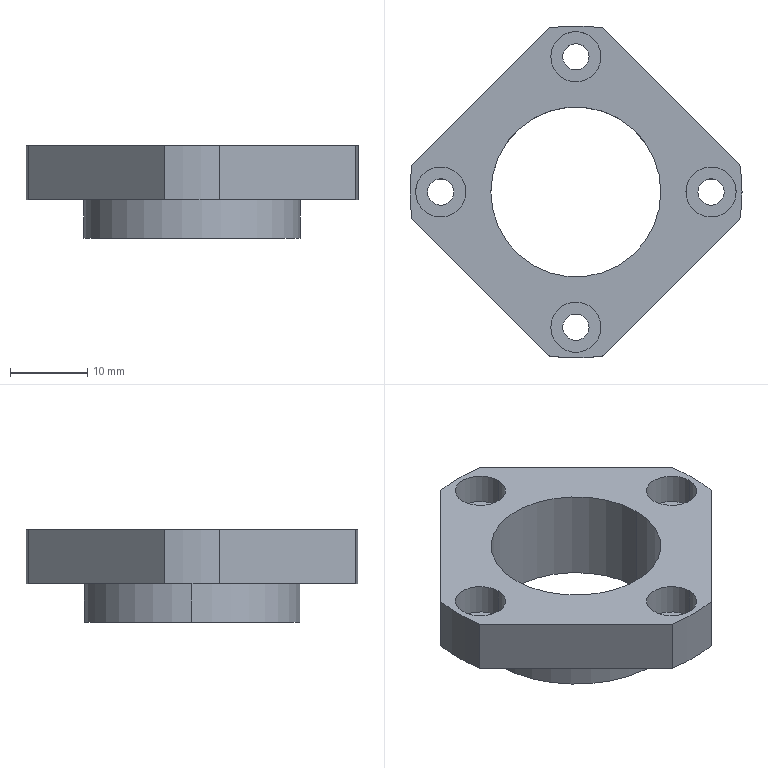Part | SolidWorks | features BaseBody 1 | 1 solid | 36 faces | box 43 x 43 x 12 mm | volume 6140 mm3 | cylinder 25 | plane 11 | commonest cylinder face diameters 3.4 x8 6.5 x8 43 x5 22 x2 28 x2
STEP:
#1=CARTESIAN_POINT('',(-11.,0.,-12.));
#2=VERTEX_POINT('',#1);
#3=CARTESIAN_POINT('',(11.,0.,-12.));
#4=VERTEX_POINT('',#3);
#5=CARTESIAN_POINT('',(0.,0.,-12.));
#6=DIRECTION('',(0.,0.,1.));
#7=DIRECTION('',(1.,0.,0.));
#8=AXIS2_PLACEMENT_3D('',#5,#6,#7);
#9=CIRCLE('',#8,11.);
#10=EDGE_CURVE('',#2,#4,#9,.T.);
#11=ORIENTED_EDGE('',*,*,#10,.F.);
#12=CARTESIAN_POINT('',(-11.,0.,0.));
#13=VERTEX_POINT('',#12);
#14=CARTESIAN_POINT('',(-11.,0.,-50.));
#15=DIRECTION('',(0.,0.,1.));
#16=VECTOR('',#15,1000.);
#17=LINE('',#14,#16);
#18=EDGE_CURVE('',#2,#13,#17,.T.);
#19=ORIENTED_EDGE('',*,*,#18,.T.);
#20=CARTESIAN_POINT('',(11.,0.,0.));
#21=VERTEX_POINT('',#20);
#22=CARTESIAN_POINT('',(0.,0.,0.));
#23=DIRECTION('',(0.,0.,-1.));
#24=DIRECTION('',(1.,0.,0.));
#25=AXIS2_PLACEMENT_3D('',#22,#23,#24);
#26=CIRCLE('',#25,11.);
#27=EDGE_CURVE('',#21,#13,#26,.T.);
#28=ORIENTED_EDGE('',*,*,#27,.F.);
#29=CARTESIAN_POINT('',(11.,0.,-50.));
#30=DIRECTION('',(0.,0.,1.));
#31=VECTOR('',#30,1000.);
#32=LINE('',#29,#31);
#33=EDGE_CURVE('',#4,#21,#32,.T.);
#34=ORIENTED_EDGE('',*,*,#33,.F.);
#35=EDGE_LOOP('',(#11,#19,#28,#34));
#36=FACE_OUTER_BOUND('',#35,.T.);
#37=CARTESIAN_POINT('',(0.,0.,-50.));
#38=DIRECTION('',(0.,0.,1.));
#39=DIRECTION('',(1.,0.,0.));
#40=AXIS2_PLACEMENT_3D('',#37,#38,#39);
#41=CYLINDRICAL_SURFACE('',#40,11.);
#42=ADVANCED_FACE('',(#36),#41,.F.);
#43=CARTESIAN_POINT('',(3.25,-17.5,0.));
#44=VERTEX_POINT('',#43);
#45=CARTESIAN_POINT('',(-3.25,-17.5,0.));
#46=VERTEX_POINT('',#45);
#47=CARTESIAN_POINT('',(0.,-17.5,0.));
#48=DIRECTION('',(0.,0.,-1.));
#49=DIRECTION('',(-1.,0.,0.));
#50=AXIS2_PLACEMENT_3D('',#47,#48,#49);
#51=CIRCLE('',#50,3.25);
#52=EDGE_CURVE('',#44,#46,#51,.T.);
#53=ORIENTED_EDGE('',*,*,#52,.F.);
#54=CARTESIAN_POINT('',(3.25,-17.5,-4.));
#55=VERTEX_POINT('',#54);
#56=CARTESIAN_POINT('',(3.25,-17.5,0.));
#57=DIRECTION('',(0.,0.,-1.));
#58=VECTOR('',#57,1000.);
#59=LINE('',#56,#58);
#60=EDGE_CURVE('',#44,#55,#59,.T.);
#61=ORIENTED_EDGE('',*,*,#60,.T.);
#62=CARTESIAN_POINT('',(-3.25,-17.5,-4.));
#63=VERTEX_POINT('',#62);
#64=CARTESIAN_POINT('',(0.,-17.5,-4.));
#65=DIRECTION('',(0.,0.,1.));
#66=DIRECTION('',(-1.,0.,0.));
#67=AXIS2_PLACEMENT_3D('',#64,#65,#66);
#68=CIRCLE('',#67,3.25);
#69=EDGE_CURVE('',#63,#55,#68,.T.);
#70=ORIENTED_EDGE('',*,*,#69,.F.);
#71=CARTESIAN_POINT('',(-3.25,-17.5,0.));
#72=DIRECTION('',(0.,0.,-1.));
#73=VECTOR('',#72,1000.);
#74=LINE('',#71,#73);
#75=EDGE_CURVE('',#46,#63,#74,.T.);
#76=ORIENTED_EDGE('',*,*,#75,.F.);
#77=EDGE_LOOP('',(#53,#61,#70,#76));
#78=FACE_OUTER_BOUND('',#77,.T.);
#79=CARTESIAN_POINT('',(0.,-17.5,0.));
#80=DIRECTION('',(0.,0.,-1.));
#81=DIRECTION('',(-1.,0.,0.));
#82=AXIS2_PLACEMENT_3D('',#79,#80,#81);
#83=CYLINDRICAL_SURFACE('',#82,3.25);
#84=ADVANCED_FACE('',(#78),#83,.F.);
#85=CARTESIAN_POINT('',(20.75,0.,0.));
#86=VERTEX_POINT('',#85);
#87=CARTESIAN_POINT('',(14.25,0.,0.));
#88=VERTEX_POINT('',#87);
#89=CARTESIAN_POINT('',(17.5,0.,0.));
#90=DIRECTION('',(0.,0.,-1.));
#91=DIRECTION('',(-1.,0.,0.));
#92=AXIS2_PLACEMENT_3D('',#89,#90,#91);
#93=CIRCLE('',#92,3.25);
#94=EDGE_CURVE('',#86,#88,#93,.T.);
#95=ORIENTED_EDGE('',*,*,#94,.F.);
#96=CARTESIAN_POINT('',(20.75,0.,-4.));
#97=VERTEX_POINT('',#96);
#98=CARTESIAN_POINT('',(20.75,0.,0.));
#99=DIRECTION('',(0.,0.,-1.));
#100=VECTOR('',#99,1000.);
#101=LINE('',#98,#100);
#102=EDGE_CURVE('',#86,#97,#101,.T.);
#103=ORIENTED_EDGE('',*,*,#102,.T.);
#104=CARTESIAN_POINT('',(14.25,0.,-4.));
#105=VERTEX_POINT('',#104);
#106=CARTESIAN_POINT('',(17.5,0.,-4.));
#107=DIRECTION('',(0.,0.,1.));
#108=DIRECTION('',(-1.,0.,0.));
#109=AXIS2_PLACEMENT_3D('',#106,#107,#108);
#110=CIRCLE('',#109,3.25);
#111=EDGE_CURVE('',#105,#97,#110,.T.);
#112=ORIENTED_EDGE('',*,*,#111,.F.);
#113=CARTESIAN_POINT('',(14.25,0.,0.));
#114=DIRECTION('',(0.,0.,-1.));
#115=VECTOR('',#114,1000.);
#116=LINE('',#113,#115);
#117=EDGE_CURVE('',#88,#105,#116,.T.);
#118=ORIENTED_EDGE('',*,*,#117,.F.);
#119=EDGE_LOOP('',(#95,#103,#112,#118));
#120=FACE_OUTER_BOUND('',#119,.T.);
#121=CARTESIAN_POINT('',(17.5,0.,0.));
#122=DIRECTION('',(0.,0.,-1.));
#123=DIRECTION('',(-1.,0.,0.));
#124=AXIS2_PLACEMENT_3D('',#121,#122,#123);
#125=CYLINDRICAL_SURFACE('',#124,3.25);
#126=ADVANCED_FACE('',(#120),#125,.F.);
#127=CARTESIAN_POINT('',(-20.75,0.,-4.));
#128=VERTEX_POINT('',#127);
#129=CARTESIAN_POINT('',(-14.25,0.,-4.));
#130=VERTEX_POINT('',#129);
#131=CARTESIAN_POINT('',(-17.5,0.,-4.));
#132=DIRECTION('',(0.,0.,1.));
#133=DIRECTION('',(1.,0.,0.));
#134=AXIS2_PLACEMENT_3D('',#131,#132,#133);
#135=CIRCLE('',#134,3.25);
#136=EDGE_CURVE('',#128,#130,#135,.T.);
#137=ORIENTED_EDGE('',*,*,#136,.F.);
#138=CARTESIAN_POINT('',(-20.75,0.,0.));
#139=VERTEX_POINT('',#138);
#140=CARTESIAN_POINT('',(-20.75,0.,-7.));
#141=DIRECTION('',(0.,0.,1.));
#142=VECTOR('',#141,1000.);
#143=LINE('',#140,#142);
#144=EDGE_CURVE('',#128,#139,#143,.T.);
#145=ORIENTED_EDGE('',*,*,#144,.T.);
#146=CARTESIAN_POINT('',(-14.25,0.,0.));
#147=VERTEX_POINT('',#146);
#148=CARTESIAN_POINT('',(-17.5,0.,0.));
#149=DIRECTION('',(0.,0.,-1.));
#150=DIRECTION('',(1.,0.,0.));
#151=AXIS2_PLACEMENT_3D('',#148,#149,#150);
#152=CIRCLE('',#151,3.25);
#153=EDGE_CURVE('',#147,#139,#152,.T.);
#154=ORIENTED_EDGE('',*,*,#153,.F.);
#155=CARTESIAN_POINT('',(-14.25,0.,-7.));
#156=DIRECTION('',(0.,0.,1.));
#157=VECTOR('',#156,1000.);
#158=LINE('',#155,#157);
#159=EDGE_CURVE('',#130,#147,#158,.T.);
#160=ORIENTED_EDGE('',*,*,#159,.F.);
#161=EDGE_LOOP('',(#137,#145,#154,#160));
#162=FACE_OUTER_BOUND('',#161,.T.);
#163=CARTESIAN_POINT('',(-17.5,0.,-7.));
#164=DIRECTION('',(0.,0.,1.));
#165=DIRECTION('',(1.,0.,0.));
#166=AXIS2_PLACEMENT_3D('',#163,#164,#165);
#167=CYLINDRICAL_SURFACE('',#166,3.25);
#168=ADVANCED_FACE('',(#162),#167,.F.);
#169=CARTESIAN_POINT('',(21.206,-3.543,-7.));
#170=VERTEX_POINT('',#169);
#171=CARTESIAN_POINT('',(21.5,0.,-7.));
#172=VERTEX_POINT('',#171);
#173=CARTESIAN_POINT('',(0.,0.,-7.));
#174=DIRECTION('',(0.,0.,1.));
#175=DIRECTION('',(1.,0.,0.));
#176=AXIS2_PLACEMENT_3D('',#173,#174,#175);
#177=CIRCLE('',#176,21.5);
#178=EDGE_CURVE('',#170,#172,#177,.T.);
#179=ORIENTED_EDGE('',*,*,#178,.T.);
#180=CARTESIAN_POINT('',(21.5,0.,0.));
#181=VERTEX_POINT('',#180);
#182=CARTESIAN_POINT('',(21.5,0.,-50.));
#183=DIRECTION('',(0.,0.,1.));
#184=VECTOR('',#183,1000.);
#185=LINE('',#182,#184);
#186=EDGE_CURVE('',#172,#181,#185,.T.);
#187=ORIENTED_EDGE('',*,*,#186,.T.);
#188=CARTESIAN_POINT('',(21.206,-3.543,0.));
#189=VERTEX_POINT('',#188);
#190=CARTESIAN_POINT('',(0.,0.,0.));
#191=DIRECTION('',(0.,0.,1.));
#192=DIRECTION('',(1.,0.,0.));
#193=AXIS2_PLACEMENT_3D('',#190,#191,#192);
#194=CIRCLE('',#193,21.5);
#195=EDGE_CURVE('',#189,#181,#194,.T.);
#196=ORIENTED_EDGE('',*,*,#195,.F.);
#197=CARTESIAN_POINT('',(21.206,-3.543,-50.));
#198=DIRECTION('',(0.,0.,-1.));
#199=VECTOR('',#198,1000.);
#200=LINE('',#197,#199);
#201=EDGE_CURVE('',#189,#170,#200,.T.);
#202=ORIENTED_EDGE('',*,*,#201,.T.);
#203=EDGE_LOOP('',(#179,#187,#196,#202));
#204=FACE_OUTER_BOUND('',#203,.T.);
#205=CARTESIAN_POINT('',(0.,0.,-50.));
#206=DIRECTION('',(0.,0.,1.));
#207=DIRECTION('',(1.,0.,0.));
#208=AXIS2_PLACEMENT_3D('',#205,#206,#207);
#209=CYLINDRICAL_SURFACE('',#208,21.5);
#210=ADVANCED_FACE('',(#204),#209,.T.);
#211=CARTESIAN_POINT('',(-3.25,17.5,-4.));
#212=VERTEX_POINT('',#211);
#213=CARTESIAN_POINT('',(3.25,17.5,-4.));
#214=VERTEX_POINT('',#213);
#215=CARTESIAN_POINT('',(0.,17.5,-4.));
#216=DIRECTION('',(0.,0.,1.));
#217=DIRECTION('',(1.,0.,0.));
#218=AXIS2_PLACEMENT_3D('',#215,#216,#217);
#219=CIRCLE('',#218,3.25);
#220=EDGE_CURVE('',#212,#214,#219,.T.);
#221=ORIENTED_EDGE('',*,*,#220,.F.);
#222=CARTESIAN_POINT('',(-3.25,17.5,0.));
#223=VERTEX_POINT('',#222);
#224=CARTESIAN_POINT('',(-3.25,17.5,-7.));
#225=DIRECTION('',(0.,0.,1.));
#226=VECTOR('',#225,1000.);
#227=LINE('',#224,#226);
#228=EDGE_CURVE('',#212,#223,#227,.T.);
#229=ORIENTED_EDGE('',*,*,#228,.T.);
#230=CARTESIAN_POINT('',(3.25,17.5,0.));
#231=VERTEX_POINT('',#230);
#232=CARTESIAN_POINT('',(0.,17.5,0.));
#233=DIRECTION('',(0.,0.,-1.));
#234=DIRECTION('',(1.,0.,0.));
#235=AXIS2_PLACEMENT_3D('',#232,#233,#234);
#236=CIRCLE('',#235,3.25);
#237=EDGE_CURVE('',#231,#223,#236,.T.);
#238=ORIENTED_EDGE('',*,*,#237,.F.);
#239=CARTESIAN_POINT('',(3.25,17.5,-7.));
#240=DIRECTION('',(0.,0.,1.));
#241=VECTOR('',#240,1000.);
#242=LINE('',#239,#241);
#243=EDGE_CURVE('',#214,#231,#242,.T.);
#244=ORIENTED_EDGE('',*,*,#243,.F.);
#245=EDGE_LOOP('',(#221,#229,#238,#244));
#246=FACE_OUTER_BOUND('',#245,.T.);
#247=CARTESIAN_POINT('',(0.,17.5,-7.));
#248=DIRECTION('',(0.,0.,1.));
#249=DIRECTION('',(1.,0.,0.));
#250=AXIS2_PLACEMENT_3D('',#247,#248,#249);
#251=CYLINDRICAL_SURFACE('',#250,3.25);
#252=ADVANCED_FACE('',(#246),#251,.F.);
#253=CARTESIAN_POINT('',(-14.,0.,-12.));
#254=VERTEX_POINT('',#253);
#255=CARTESIAN_POINT('',(14.,0.,-12.));
#256=VERTEX_POINT('',#255);
#257=CARTESIAN_POINT('',(0.,0.,-12.));
#258=DIRECTION('',(0.,0.,-1.));
#259=DIRECTION('',(1.,0.,0.));
#260=AXIS2_PLACEMENT_3D('',#257,#258,#259);
#261=CIRCLE('',#260,14.);
#262=EDGE_CURVE('',#254,#256,#261,.T.);
#263=ORIENTED_EDGE('',*,*,#262,.F.);
#264=CARTESIAN_POINT('',(-14.,0.,-7.));
#265=VERTEX_POINT('',#264);
#266=CARTESIAN_POINT('',(-14.,0.,-50.));
#267=DIRECTION('',(0.,0.,1.));
#268=VECTOR('',#267,1000.);
#269=LINE('',#266,#268);
#270=EDGE_CURVE('',#254,#265,#269,.T.);
#271=ORIENTED_EDGE('',*,*,#270,.T.);
#272=CARTESIAN_POINT('',(14.,0.,-7.));
#273=VERTEX_POINT('',#272);
#274=CARTESIAN_POINT('',(0.,0.,-7.));
#275=DIRECTION('',(0.,0.,-1.));
#276=DIRECTION('',(1.,0.,0.));
#277=AXIS2_PLACEMENT_3D('',#274,#275,#276);
#278=CIRCLE('',#277,14.);
#279=EDGE_CURVE('',#265,#273,#278,.T.);
#280=ORIENTED_EDGE('',*,*,#279,.T.);
#281=CARTESIAN_POINT('',(14.,0.,-50.));
#282=DIRECTION('',(0.,0.,1.));
#283=VECTOR('',#282,1000.);
#284=LINE('',#281,#283);
#285=EDGE_CURVE('',#256,#273,#284,.T.);
#286=ORIENTED_EDGE('',*,*,#285,.F.);
#287=EDGE_LOOP('',(#263,#271,#280,#286));
#288=FACE_OUTER_BOUND('',#287,.T.);
#289=CARTESIAN_POINT('',(0.,0.,-50.));
#290=DIRECTION('',(0.,0.,1.));
#291=DIRECTION('',(1.,0.,0.));
#292=AXIS2_PLACEMENT_3D('',#289,#290,#291);
#293=CYLINDRICAL_SURFACE('',#292,14.);
#294=ADVANCED_FACE('',(#288),#293,.T.);
#295=CARTESIAN_POINT('',(1.7,-17.5,-4.));
#296=VERTEX_POINT('',#295);
#297=CARTESIAN_POINT('',(-1.7,-17.5,-4.));
#298=VERTEX_POINT('',#297);
#299=CARTESIAN_POINT('',(0.,-17.5,-4.));
#300=DIRECTION('',(0.,0.,-1.));
#301=DIRECTION('',(-1.,0.,0.));
#302=AXIS2_PLACEMENT_3D('',#299,#300,#301);
#303=CIRCLE('',#302,1.7);
#304=EDGE_CURVE('',#296,#298,#303,.T.);
#305=ORIENTED_EDGE('',*,*,#304,.F.);
#306=CARTESIAN_POINT('',(1.7,-17.5,-7.));
#307=VERTEX_POINT('',#306);
#308=CARTESIAN_POINT('',(1.7,-17.5,0.));
#309=DIRECTION('',(0.,0.,-1.));
#310=VECTOR('',#309,1000.);
#311=LINE('',#308,#310);
#312=EDGE_CURVE('',#296,#307,#311,.T.);
#313=ORIENTED_EDGE('',*,*,#312,.T.);
#314=CARTESIAN_POINT('',(-1.7,-17.5,-7.));
#315=VERTEX_POINT('',#314);
#316=CARTESIAN_POINT('',(0.,-17.5,-7.));
#317=DIRECTION('',(0.,0.,1.));
#318=DIRECTION('',(-1.,0.,0.));
#319=AXIS2_PLACEMENT_3D('',#316,#317,#318);
#320=CIRCLE('',#319,1.7);
#321=EDGE_CURVE('',#315,#307,#320,.T.);
#322=ORIENTED_EDGE('',*,*,#321,.F.);
#323=CARTESIAN_POINT('',(-1.7,-17.5,0.));
#324=DIRECTION('',(0.,0.,-1.));
#325=VECTOR('',#324,1000.);
#326=LINE('',#323,#325);
#327=EDGE_CURVE('',#298,#315,#326,.T.);
#328=ORIENTED_EDGE('',*,*,#327,.F.);
#329=EDGE_LOOP('',(#305,#313,#322,#328));
#330=FACE_OUTER_BOUND('',#329,.T.);
#331=CARTESIAN_POINT('',(0.,-17.5,0.));
#332=DIRECTION('',(0.,0.,-1.));
#333=DIRECTION('',(-1.,0.,0.));
#334=AXIS2_PLACEMENT_3D('',#331,#332,#333);
#335=CYLINDRICAL_SURFACE('',#334,1.7);
#336=ADVANCED_FACE('',(#330),#335,.F.);
#337=CARTESIAN_POINT('',(19.2,0.,-4.));
#338=VERTEX_POINT('',#337);
#339=CARTESIAN_POINT('',(15.8,0.,-4.));
#340=VERTEX_POINT('',#339);
#341=CARTESIAN_POINT('',(17.5,0.,-4.));
#342=DIRECTION('',(0.,0.,-1.));
#343=DIRECTION('',(-1.,0.,0.));
#344=AXIS2_PLACEMENT_3D('',#341,#342,#343);
#345=CIRCLE('',#344,1.7);
#346=EDGE_CURVE('',#338,#340,#345,.T.);
#347=ORIENTED_EDGE('',*,*,#346,.F.);
#348=CARTESIAN_POINT('',(19.2,0.,-7.));
#349=VERTEX_POINT('',#348);
#350=CARTESIAN_POINT('',(19.2,0.,0.));
#351=DIRECTION('',(0.,0.,-1.));
#352=VECTOR('',#351,1000.);
#353=LINE('',#350,#352);
#354=EDGE_CURVE('',#338,#349,#353,.T.);
#355=ORIENTED_EDGE('',*,*,#354,.T.);
#356=CARTESIAN_POINT('',(15.8,0.,-7.));
#357=VERTEX_POINT('',#356);
#358=CARTESIAN_POINT('',(17.5,0.,-7.));
#359=DIRECTION('',(0.,0.,1.));
#360=DIRECTION('',(-1.,0.,0.));
#361=AXIS2_PLACEMENT_3D('',#358,#359,#360);
#362=CIRCLE('',#361,1.7);
#363=EDGE_CURVE('',#357,#349,#362,.T.);
#364=ORIENTED_EDGE('',*,*,#363,.F.);
#365=CARTESIAN_POINT('',(15.8,0.,0.));
#366=DIRECTION('',(0.,0.,-1.));
#367=VECTOR('',#366,1000.);
#368=LINE('',#365,#367);
#369=EDGE_CURVE('',#340,#357,#368,.T.);
#370=ORIENTED_EDGE('',*,*,#369,.F.);
#371=EDGE_LOOP('',(#347,#355,#364,#370));
#372=FACE_OUTER_BOUND('',#371,.T.);
#373=CARTESIAN_POINT('',(17.5,0.,0.));
#374=DIRECTION('',(0.,0.,-1.));
#375=DIRECTION('',(-1.,0.,0.));
#376=AXIS2_PLACEMENT_3D('',#373,#374,#375);
#377=CYLINDRICAL_SURFACE('',#376,1.7);
#378=ADVANCED_FACE('',(#372),#377,.F.);
#379=CARTESIAN_POINT('',(-19.2,0.,-7.));
#380=VERTEX_POINT('',#379);
#381=CARTESIAN_POINT('',(-15.8,0.,-7.));
#382=VERTEX_POINT('',#381);
#383=CARTESIAN_POINT('',(-17.5,0.,-7.));
#384=DIRECTION('',(0.,0.,1.));
#385=DIRECTION('',(1.,0.,0.));
#386=AXIS2_PLACEMENT_3D('',#383,#384,#385);
#387=CIRCLE('',#386,1.7);
#388=EDGE_CURVE('',#380,#382,#387,.T.);
#389=ORIENTED_EDGE('',*,*,#388,.F.);
#390=CARTESIAN_POINT('',(-19.2,0.,-4.));
#391=VERTEX_POINT('',#390);
#392=CARTESIAN_POINT('',(-19.2,0.,-7.));
#393=DIRECTION('',(0.,0.,1.));
#394=VECTOR('',#393,1000.);
#395=LINE('',#392,#394);
#396=EDGE_CURVE('',#380,#391,#395,.T.);
#397=ORIENTED_EDGE('',*,*,#396,.T.);
#398=CARTESIAN_POINT('',(-15.8,0.,-4.));
#399=VERTEX_POINT('',#398);
#400=CARTESIAN_POINT('',(-17.5,0.,-4.));
#401=DIRECTION('',(0.,0.,-1.));
#402=DIRECTION('',(1.,0.,0.));
#403=AXIS2_PLACEMENT_3D('',#400,#401,#402);
#404=CIRCLE('',#403,1.7);
#405=EDGE_CURVE('',#399,#391,#404,.T.);
#406=ORIENTED_EDGE('',*,*,#405,.F.);
#407=CARTESIAN_POINT('',(-15.8,0.,-7.));
#408=DIRECTION('',(0.,0.,1.));
#409=VECTOR('',#408,1000.);
#410=LINE('',#407,#409);
#411=EDGE_CURVE('',#382,#399,#410,.T.);
#412=ORIENTED_EDGE('',*,*,#411,.F.);
#413=EDGE_LOOP('',(#389,#397,#406,#412));
#414=FACE_OUTER_BOUND('',#413,.T.);
#415=CARTESIAN_POINT('',(-17.5,0.,-7.));
#416=DIRECTION('',(0.,0.,1.));
#417=DIRECTION('',(1.,0.,0.));
#418=AXIS2_PLACEMENT_3D('',#415,#416,#417);
#419=CYLINDRICAL_SURFACE('',#418,1.7);
#420=ADVANCED_FACE('',(#414),#419,.F.);
#421=CARTESIAN_POINT('',(-1.7,17.5,-7.));
#422=VERTEX_POINT('',#421);
#423=CARTESIAN_POINT('',(1.7,17.5,-7.));
#424=VERTEX_POINT('',#423);
#425=CARTESIAN_POINT('',(0.,17.5,-7.));
#426=DIRECTION('',(0.,0.,1.));
#427=DIRECTION('',(1.,0.,0.));
#428=AXIS2_PLACEMENT_3D('',#425,#426,#427);
#429=CIRCLE('',#428,1.7);
#430=EDGE_CURVE('',#422,#424,#429,.T.);
#431=ORIENTED_EDGE('',*,*,#430,.F.);
#432=CARTESIAN_POINT('',(-1.7,17.5,-4.));
#433=VERTEX_POINT('',#432);
#434=CARTESIAN_POINT('',(-1.7,17.5,-7.));
#435=DIRECTION('',(0.,0.,1.));
#436=VECTOR('',#435,1000.);
#437=LINE('',#434,#436);
#438=EDGE_CURVE('',#422,#433,#437,.T.);
#439=ORIENTED_EDGE('',*,*,#438,.T.);
#440=CARTESIAN_POINT('',(1.7,17.5,-4.));
#441=VERTEX_POINT('',#440);
#442=CARTESIAN_POINT('',(0.,17.5,-4.));
#443=DIRECTION('',(0.,0.,-1.));
#444=DIRECTION('',(1.,0.,0.));
#445=AXIS2_PLACEMENT_3D('',#442,#443,#444);
#446=CIRCLE('',#445,1.7);
#447=EDGE_CURVE('',#441,#433,#446,.T.);
#448=ORIENTED_EDGE('',*,*,#447,.F.);
#449=CARTESIAN_POINT('',(1.7,17.5,-7.));
#450=DIRECTION('',(0.,0.,1.));
#451=VECTOR('',#450,1000.);
#452=LINE('',#449,#451);
#453=EDGE_CURVE('',#424,#441,#452,.T.);
#454=ORIENTED_EDGE('',*,*,#453,.F.);
#455=EDGE_LOOP('',(#431,#439,#448,#454));
#456=FACE_OUTER_BOUND('',#455,.T.);
#457=CARTESIAN_POINT('',(0.,17.5,-7.));
#458=DIRECTION('',(0.,0.,1.));
#459=DIRECTION('',(1.,0.,0.));
#460=AXIS2_PLACEMENT_3D('',#457,#458,#459);
#461=CYLINDRICAL_SURFACE('',#460,1.7);
#462=ADVANCED_FACE('',(#456),#461,.F.);
#463=ORIENTED_EDGE('',*,*,#18,.F.);
#464=CARTESIAN_POINT('',(0.,0.,-12.));
#465=DIRECTION('',(0.,0.,1.));
#466=DIRECTION('',(1.,0.,0.));
#467=AXIS2_PLACEMENT_3D('',#464,#465,#466);
#468=CIRCLE('',#467,11.);
#469=EDGE_CURVE('',#4,#2,#468,.T.);
#470=ORIENTED_EDGE('',*,*,#469,.F.);
#471=ORIENTED_EDGE('',*,*,#33,.T.);
#472=CARTESIAN_POINT('',(0.,0.,0.));
#473=DIRECTION('',(0.,0.,-1.));
#474=DIRECTION('',(1.,0.,0.));
#475=AXIS2_PLACEMENT_3D('',#472,#473,#474);
#476=CIRCLE('',#475,11.);
#477=EDGE_CURVE('',#13,#21,#476,.T.);
#478=ORIENTED_EDGE('',*,*,#477,.F.);
#479=EDGE_LOOP('',(#463,#470,#471,#478));
#480=FACE_OUTER_BOUND('',#479,.T.);
#481=CARTESIAN_POINT('',(0.,0.,-50.));
#482=DIRECTION('',(0.,0.,1.));
#483=DIRECTION('',(1.,0.,0.));
#484=AXIS2_PLACEMENT_3D('',#481,#482,#483);
#485=CYLINDRICAL_SURFACE('',#484,11.);
#486=ADVANCED_FACE('',(#480),#485,.F.);
#487=CARTESIAN_POINT('',(0.,-17.5,0.));
#488=DIRECTION('',(0.,0.,-1.));
#489=DIRECTION('',(-1.,0.,0.));
#490=AXIS2_PLACEMENT_3D('',#487,#488,#489);
#491=CIRCLE('',#490,3.25);
#492=EDGE_CURVE('',#46,#44,#491,.T.);
#493=ORIENTED_EDGE('',*,*,#492,.T.);
#494=ORIENTED_EDGE('',*,*,#52,.T.);
#495=EDGE_LOOP('',(#493,#494));
#496=FACE_BOUND('',#495,.T.);
#497=CARTESIAN_POINT('',(17.5,0.,0.));
#498=DIRECTION('',(0.,0.,-1.));
#499=DIRECTION('',(-1.,0.,0.));
#500=AXIS2_PLACEMENT_3D('',#497,#498,#499);
#501=CIRCLE('',#500,3.25);
#502=EDGE_CURVE('',#88,#86,#501,.T.);
#503=ORIENTED_EDGE('',*,*,#502,.T.);
#504=ORIENTED_EDGE('',*,*,#94,.T.);
#505=EDGE_LOOP('',(#503,#504));
#506=FACE_BOUND('',#505,.T.);
#507=ORIENTED_EDGE('',*,*,#153,.T.);
#508=CARTESIAN_POINT('',(-17.5,0.,0.));
#509=DIRECTION('',(0.,0.,-1.));
#510=DIRECTION('',(1.,0.,0.));
#511=AXIS2_PLACEMENT_3D('',#508,#509,#510);
#512=CIRCLE('',#511,3.25);
#513=EDGE_CURVE('',#139,#147,#512,.T.);
#514=ORIENTED_EDGE('',*,*,#513,.T.);
#515=EDGE_LOOP('',(#507,#514));
#516=FACE_BOUND('',#515,.T.);
#517=CARTESIAN_POINT('',(-21.206,-3.543,0.));
#518=VERTEX_POINT('',#517);
#519=CARTESIAN_POINT('',(-3.543,-21.206,0.));
#520=VERTEX_POINT('',#519);
#521=CARTESIAN_POINT('',(-21.206,-3.543,0.));
#522=DIRECTION('',(0.7071,-0.7071,0.));
#523=VECTOR('',#522,1000.);
#524=LINE('',#521,#523);
#525=EDGE_CURVE('',#518,#520,#524,.T.);
#526=ORIENTED_EDGE('',*,*,#525,.T.);
#527=CARTESIAN_POINT('',(3.543,-21.206,0.));
#528=VERTEX_POINT('',#527);
#529=CARTESIAN_POINT('',(0.,0.,0.));
#530=DIRECTION('',(0.,0.,1.));
#531=DIRECTION('',(1.,0.,0.));
#532=AXIS2_PLACEMENT_3D('',#529,#530,#531);
#533=CIRCLE('',#532,21.5);
#534=EDGE_CURVE('',#520,#528,#533,.T.);
#535=ORIENTED_EDGE('',*,*,#534,.T.);
#536=CARTESIAN_POINT('',(3.543,-21.206,0.));
#537=DIRECTION('',(0.7071,0.7071,0.));
#538=VECTOR('',#537,1000.);
#539=LINE('',#536,#538);
#540=EDGE_CURVE('',#528,#189,#539,.T.);
#541=ORIENTED_EDGE('',*,*,#540,.T.);
#542=ORIENTED_EDGE('',*,*,#195,.T.);
#543=CARTESIAN_POINT('',(21.206,3.543,0.));
#544=VERTEX_POINT('',#543);
#545=CARTESIAN_POINT('',(0.,0.,0.));
#546=DIRECTION('',(0.,0.,1.));
#547=DIRECTION('',(1.,0.,0.));
#548=AXIS2_PLACEMENT_3D('',#545,#546,#547);
#549=CIRCLE('',#548,21.5);
#550=EDGE_CURVE('',#181,#544,#549,.T.);
#551=ORIENTED_EDGE('',*,*,#550,.T.);
#552=CARTESIAN_POINT('',(3.543,21.206,0.));
#553=VERTEX_POINT('',#552);
#554=CARTESIAN_POINT('',(21.206,3.543,0.));
#555=DIRECTION('',(-0.7071,0.7071,0.));
#556=VECTOR('',#555,1000.);
#557=LINE('',#554,#556);
#558=EDGE_CURVE('',#544,#553,#557,.T.);
#559=ORIENTED_EDGE('',*,*,#558,.T.);
#560=CARTESIAN_POINT('',(-3.543,21.206,0.));
#561=VERTEX_POINT('',#560);
#562=CARTESIAN_POINT('',(0.,0.,0.));
#563=DIRECTION('',(0.,0.,1.));
#564=DIRECTION('',(1.,0.,0.));
#565=AXIS2_PLACEMENT_3D('',#562,#563,#564);
#566=CIRCLE('',#565,21.5);
#567=EDGE_CURVE('',#553,#561,#566,.T.);
#568=ORIENTED_EDGE('',*,*,#567,.T.);
#569=CARTESIAN_POINT('',(-21.206,3.543,0.));
#570=VERTEX_POINT('',#569);
#571=CARTESIAN_POINT('',(-3.543,21.206,0.));
#572=DIRECTION('',(-0.7071,-0.7071,0.));
#573=VECTOR('',#572,1000.);
#574=LINE('',#571,#573);
#575=EDGE_CURVE('',#561,#570,#574,.T.);
#576=ORIENTED_EDGE('',*,*,#575,.T.);
#577=CARTESIAN_POINT('',(0.,0.,0.));
#578=DIRECTION('',(0.,0.,1.));
#579=DIRECTION('',(1.,0.,0.));
#580=AXIS2_PLACEMENT_3D('',#577,#578,#579);
#581=CIRCLE('',#580,21.5);
#582=EDGE_CURVE('',#570,#518,#581,.T.);
#583=ORIENTED_EDGE('',*,*,#582,.T.);
#584=EDGE_LOOP('',(#526,#535,#541,#542,#551,#559,#568,#576,#583));
#585=FACE_OUTER_BOUND('',#584,.T.);
#586=ORIENTED_EDGE('',*,*,#237,.T.);
#587=CARTESIAN_POINT('',(0.,17.5,0.));
#588=DIRECTION('',(0.,0.,-1.));
#589=DIRECTION('',(1.,0.,0.));
#590=AXIS2_PLACEMENT_3D('',#587,#588,#589);
#591=CIRCLE('',#590,3.25);
#592=EDGE_CURVE('',#223,#231,#591,.T.);
#593=ORIENTED_EDGE('',*,*,#592,.T.);
#594=EDGE_LOOP('',(#586,#593));
#595=FACE_BOUND('',#594,.T.);
#596=ORIENTED_EDGE('',*,*,#27,.T.);
#597=ORIENTED_EDGE('',*,*,#477,.T.);
#598=EDGE_LOOP('',(#596,#597));
#599=FACE_BOUND('',#598,.T.);
#600=CARTESIAN_POINT('',(0.,21.5,0.));
#601=DIRECTION('',(0.,0.,1.));
#602=DIRECTION('',(1.,0.,0.));
#603=AXIS2_PLACEMENT_3D('',#600,#601,#602);
#604=PLANE('',#603);
#605=ADVANCED_FACE('',(#496,#506,#516,#585,#595,#599),#604,.T.);
#606=ORIENTED_EDGE('',*,*,#469,.T.);
#607=ORIENTED_EDGE('',*,*,#10,.T.);
#608=EDGE_LOOP('',(#606,#607));
#609=FACE_BOUND('',#608,.T.);
#610=CARTESIAN_POINT('',(0.,0.,-12.));
#611=DIRECTION('',(0.,0.,-1.));
#612=DIRECTION('',(1.,0.,0.));
#613=AXIS2_PLACEMENT_3D('',#610,#611,#612);
#614=CIRCLE('',#613,14.);
#615=EDGE_CURVE('',#256,#254,#614,.T.);
#616=ORIENTED_EDGE('',*,*,#615,.T.);
#617=ORIENTED_EDGE('',*,*,#262,.T.);
#618=EDGE_LOOP('',(#616,#617));
#619=FACE_OUTER_BOUND('',#618,.T.);
#620=CARTESIAN_POINT('',(0.,11.,-12.));
#621=DIRECTION('',(0.,0.,-1.));
#622=DIRECTION('',(-1.,0.,0.));
#623=AXIS2_PLACEMENT_3D('',#620,#621,#622);
#624=PLANE('',#623);
#625=ADVANCED_FACE('',(#609,#619),#624,.T.);
#626=ORIENTED_EDGE('',*,*,#60,.F.);
#627=ORIENTED_EDGE('',*,*,#492,.F.);
#628=ORIENTED_EDGE('',*,*,#75,.T.);
#629=CARTESIAN_POINT('',(0.,-17.5,-4.));
#630=DIRECTION('',(0.,0.,1.));
#631=DIRECTION('',(-1.,0.,0.));
#632=AXIS2_PLACEMENT_3D('',#629,#630,#631);
#633=CIRCLE('',#632,3.25);
#634=EDGE_CURVE('',#55,#63,#633,.T.);
#635=ORIENTED_EDGE('',*,*,#634,.F.);
#636=EDGE_LOOP('',(#626,#627,#628,#635));
#637=FACE_OUTER_BOUND('',#636,.T.);
#638=CARTESIAN_POINT('',(0.,-17.5,0.));
#639=DIRECTION('',(0.,0.,-1.));
#640=DIRECTION('',(-1.,0.,0.));
#641=AXIS2_PLACEMENT_3D('',#638,#639,#640);
#642=CYLINDRICAL_SURFACE('',#641,3.25);
#643=ADVANCED_FACE('',(#637),#642,.F.);
#644=ORIENTED_EDGE('',*,*,#102,.F.);
#645=ORIENTED_EDGE('',*,*,#502,.F.);
#646=ORIENTED_EDGE('',*,*,#117,.T.);
#647=CARTESIAN_POINT('',(17.5,0.,-4.));
#648=DIRECTION('',(0.,0.,1.));
#649=DIRECTION('',(-1.,0.,0.));
#650=AXIS2_PLACEMENT_3D('',#647,#648,#649);
#651=CIRCLE('',#650,3.25);
#652=EDGE_CURVE('',#97,#105,#651,.T.);
#653=ORIENTED_EDGE('',*,*,#652,.F.);
#654=EDGE_LOOP('',(#644,#645,#646,#653));
#655=FACE_OUTER_BOUND('',#654,.T.);
#656=CARTESIAN_POINT('',(17.5,0.,0.));
#657=DIRECTION('',(0.,0.,-1.));
#658=DIRECTION('',(-1.,0.,0.));
#659=AXIS2_PLACEMENT_3D('',#656,#657,#658);
#660=CYLINDRICAL_SURFACE('',#659,3.25);
#661=ADVANCED_FACE('',(#655),#660,.F.);
#662=ORIENTED_EDGE('',*,*,#144,.F.);
#663=CARTESIAN_POINT('',(-17.5,0.,-4.));
#664=DIRECTION('',(0.,0.,1.));
#665=DIRECTION('',(1.,0.,0.));
#666=AXIS2_PLACEMENT_3D('',#663,#664,#665);
#667=CIRCLE('',#666,3.25);
#668=EDGE_CURVE('',#130,#128,#667,.T.);
#669=ORIENTED_EDGE('',*,*,#668,.F.);
#670=ORIENTED_EDGE('',*,*,#159,.T.);
#671=ORIENTED_EDGE('',*,*,#513,.F.);
#672=EDGE_LOOP('',(#662,#669,#670,#671));
#673=FACE_OUTER_BOUND('',#672,.T.);
#674=CARTESIAN_POINT('',(-17.5,0.,-7.));
#675=DIRECTION('',(0.,0.,1.));
#676=DIRECTION('',(1.,0.,0.));
#677=AXIS2_PLACEMENT_3D('',#674,#675,#676);
#678=CYLINDRICAL_SURFACE('',#677,3.25);
#679=ADVANCED_FACE('',(#673),#678,.F.);
#680=CARTESIAN_POINT('',(-3.543,-21.206,-7.));
#681=VERTEX_POINT('',#680);
#682=CARTESIAN_POINT('',(-3.543,-21.206,-50.));
#683=DIRECTION('',(0.,0.,-1.));
#684=VECTOR('',#683,1000.);
#685=LINE('',#682,#684);
#686=EDGE_CURVE('',#520,#681,#685,.T.);
#687=ORIENTED_EDGE('',*,*,#686,.T.);
#688=CARTESIAN_POINT('',(3.543,-21.206,-7.));
#689=VERTEX_POINT('',#688);
#690=CARTESIAN_POINT('',(0.,0.,-7.));
#691=DIRECTION('',(0.,0.,1.));
#692=DIRECTION('',(1.,0.,0.));
#693=AXIS2_PLACEMENT_3D('',#690,#691,#692);
#694=CIRCLE('',#693,21.5);
#695=EDGE_CURVE('',#681,#689,#694,.T.);
#696=ORIENTED_EDGE('',*,*,#695,.T.);
#697=CARTESIAN_POINT('',(3.543,-21.206,-50.));
#698=DIRECTION('',(0.,0.,1.));
#699=VECTOR('',#698,1000.);
#700=LINE('',#697,#699);
#701=EDGE_CURVE('',#689,#528,#700,.T.);
#702=ORIENTED_EDGE('',*,*,#701,.T.);
#703=ORIENTED_EDGE('',*,*,#534,.F.);
#704=EDGE_LOOP('',(#687,#696,#702,#703));
#705=FACE_OUTER_BOUND('',#704,.T.);
#706=CARTESIAN_POINT('',(0.,0.,-50.));
#707=DIRECTION('',(0.,0.,1.));
#708=DIRECTION('',(1.,0.,0.));
#709=AXIS2_PLACEMENT_3D('',#706,#707,#708);
#710=CYLINDRICAL_SURFACE('',#709,21.5);
#711=ADVANCED_FACE('',(#705),#710,.T.);
#712=CARTESIAN_POINT('',(-21.206,-3.543,-7.));
#713=VERTEX_POINT('',#712);
#714=CARTESIAN_POINT('',(-21.206,-3.543,-7.));
#715=DIRECTION('',(0.,0.,1.));
#716=VECTOR('',#715,1000.);
#717=LINE('',#714,#716);
#718=EDGE_CURVE('',#713,#518,#717,.T.);
#719=ORIENTED_EDGE('',*,*,#718,.F.);
#720=CARTESIAN_POINT('',(-3.543,-21.206,-7.));
#721=DIRECTION('',(-0.7071,0.7071,0.));
#722=VECTOR('',#721,1000.);
#723=LINE('',#720,#722);
#724=EDGE_CURVE('',#681,#713,#723,.T.);
#725=ORIENTED_EDGE('',*,*,#724,.F.);
#726=ORIENTED_EDGE('',*,*,#686,.F.);
#727=ORIENTED_EDGE('',*,*,#525,.F.);
#728=EDGE_LOOP('',(#719,#725,#726,#727));
#729=FACE_OUTER_BOUND('',#728,.T.);
#730=CARTESIAN_POINT('',(-3.543,-21.206,-7.));
#731=DIRECTION('',(0.7071,0.7071,0.));
#732=DIRECTION('',(-0.7071,0.7071,0.));
#733=AXIS2_PLACEMENT_3D('',#730,#731,#732);
#734=PLANE('',#733);
#735=ADVANCED_FACE('',(#729),#734,.F.);
#736=CARTESIAN_POINT('',(-21.206,3.543,-7.));
#737=VERTEX_POINT('',#736);
#738=CARTESIAN_POINT('',(-21.206,3.543,-50.));
#739=DIRECTION('',(0.,0.,-1.));
#740=VECTOR('',#739,1000.);
#741=LINE('',#738,#740);
#742=EDGE_CURVE('',#570,#737,#741,.T.);
#743=ORIENTED_EDGE('',*,*,#742,.T.);
#744=CARTESIAN_POINT('',(0.,0.,-7.));
#745=DIRECTION('',(0.,0.,1.));
#746=DIRECTION('',(1.,0.,0.));
#747=AXIS2_PLACEMENT_3D('',#744,#745,#746);
#748=CIRCLE('',#747,21.5);
#749=EDGE_CURVE('',#737,#713,#748,.T.);
#750=ORIENTED_EDGE('',*,*,#749,.T.);
#751=ORIENTED_EDGE('',*,*,#718,.T.);
#752=ORIENTED_EDGE('',*,*,#582,.F.);
#753=EDGE_LOOP('',(#743,#750,#751,#752));
#754=FACE_OUTER_BOUND('',#753,.T.);
#755=CARTESIAN_POINT('',(0.,0.,-50.));
#756=DIRECTION('',(0.,0.,1.));
#757=DIRECTION('',(1.,0.,0.));
#758=AXIS2_PLACEMENT_3D('',#755,#756,#757);
#759=CYLINDRICAL_SURFACE('',#758,21.5);
#760=ADVANCED_FACE('',(#754),#759,.T.);
#761=CARTESIAN_POINT('',(-3.543,21.206,-7.));
#762=VERTEX_POINT('',#761);
#763=CARTESIAN_POINT('',(-3.543,21.206,-7.));
#764=DIRECTION('',(0.,0.,1.));
#765=VECTOR('',#764,1000.);
#766=LINE('',#763,#765);
#767=EDGE_CURVE('',#762,#561,#766,.T.);
#768=ORIENTED_EDGE('',*,*,#767,.F.);
#769=CARTESIAN_POINT('',(-21.206,3.543,-7.));
#770=DIRECTION('',(0.7071,0.7071,0.));
#771=VECTOR('',#770,1000.);
#772=LINE('',#769,#771);
#773=EDGE_CURVE('',#737,#762,#772,.T.);
#774=ORIENTED_EDGE('',*,*,#773,.F.);
#775=ORIENTED_EDGE('',*,*,#742,.F.);
#776=ORIENTED_EDGE('',*,*,#575,.F.);
#777=EDGE_LOOP('',(#768,#774,#775,#776));
#778=FACE_OUTER_BOUND('',#777,.T.);
#779=CARTESIAN_POINT('',(-21.206,3.543,-7.));
#780=DIRECTION('',(0.7071,-0.7071,0.));
#781=DIRECTION('',(0.7071,0.7071,0.));
#782=AXIS2_PLACEMENT_3D('',#779,#780,#781);
#783=PLANE('',#782);
#784=ADVANCED_FACE('',(#778),#783,.F.);
#785=CARTESIAN_POINT('',(3.543,21.206,-7.));
#786=VERTEX_POINT('',#785);
#787=CARTESIAN_POINT('',(3.543,21.206,-50.));
#788=DIRECTION('',(0.,0.,-1.));
#789=VECTOR('',#788,1000.);
#790=LINE('',#787,#789);
#791=EDGE_CURVE('',#553,#786,#790,.T.);
#792=ORIENTED_EDGE('',*,*,#791,.T.);
#793=CARTESIAN_POINT('',(0.,0.,-7.));
#794=DIRECTION('',(0.,0.,1.));
#795=DIRECTION('',(1.,0.,0.));
#796=AXIS2_PLACEMENT_3D('',#793,#794,#795);
#797=CIRCLE('',#796,21.5);
#798=EDGE_CURVE('',#786,#762,#797,.T.);
#799=ORIENTED_EDGE('',*,*,#798,.T.);
#800=ORIENTED_EDGE('',*,*,#767,.T.);
#801=ORIENTED_EDGE('',*,*,#567,.F.);
#802=EDGE_LOOP('',(#792,#799,#800,#801));
#803=FACE_OUTER_BOUND('',#802,.T.);
#804=CARTESIAN_POINT('',(0.,0.,-50.));
#805=DIRECTION('',(0.,0.,1.));
#806=DIRECTION('',(1.,0.,0.));
#807=AXIS2_PLACEMENT_3D('',#804,#805,#806);
#808=CYLINDRICAL_SURFACE('',#807,21.5);
#809=ADVANCED_FACE('',(#803),#808,.T.);
#810=CARTESIAN_POINT('',(21.206,3.543,-7.));
#811=VERTEX_POINT('',#810);
#812=CARTESIAN_POINT('',(21.206,3.543,-7.));
#813=DIRECTION('',(0.,0.,1.));
#814=VECTOR('',#813,1000.);
#815=LINE('',#812,#814);
#816=EDGE_CURVE('',#811,#544,#815,.T.);
#817=ORIENTED_EDGE('',*,*,#816,.F.);
#818=CARTESIAN_POINT('',(3.543,21.206,-7.));
#819=DIRECTION('',(0.7071,-0.7071,0.));
#820=VECTOR('',#819,1000.);
#821=LINE('',#818,#820);
#822=EDGE_CURVE('',#786,#811,#821,.T.);
#823=ORIENTED_EDGE('',*,*,#822,.F.);
#824=ORIENTED_EDGE('',*,*,#791,.F.);
#825=ORIENTED_EDGE('',*,*,#558,.F.);
#826=EDGE_LOOP('',(#817,#823,#824,#825));
#827=FACE_OUTER_BOUND('',#826,.T.);
#828=CARTESIAN_POINT('',(3.543,21.206,-7.));
#829=DIRECTION('',(-0.7071,-0.7071,0.));
#830=DIRECTION('',(0.7071,-0.7071,0.));
#831=AXIS2_PLACEMENT_3D('',#828,#829,#830);
#832=PLANE('',#831);
#833=ADVANCED_FACE('',(#827),#832,.F.);
#834=ORIENTED_EDGE('',*,*,#186,.F.);
#835=CARTESIAN_POINT('',(0.,0.,-7.));
#836=DIRECTION('',(0.,0.,1.));
#837=DIRECTION('',(1.,0.,0.));
#838=AXIS2_PLACEMENT_3D('',#835,#836,#837);
#839=CIRCLE('',#838,21.5);
#840=EDGE_CURVE('',#172,#811,#839,.T.);
#841=ORIENTED_EDGE('',*,*,#840,.T.);
#842=ORIENTED_EDGE('',*,*,#816,.T.);
#843=ORIENTED_EDGE('',*,*,#550,.F.);
#844=EDGE_LOOP('',(#834,#841,#842,#843));
#845=FACE_OUTER_BOUND('',#844,.T.);
#846=CARTESIAN_POINT('',(0.,0.,-50.));
#847=DIRECTION('',(0.,0.,1.));
#848=DIRECTION('',(1.,0.,0.));
#849=AXIS2_PLACEMENT_3D('',#846,#847,#848);
#850=CYLINDRICAL_SURFACE('',#849,21.5);
#851=ADVANCED_FACE('',(#845),#850,.T.);
#852=ORIENTED_EDGE('',*,*,#701,.F.);
#853=CARTESIAN_POINT('',(21.206,-3.543,-7.));
#854=DIRECTION('',(-0.7071,-0.7071,0.));
#855=VECTOR('',#854,1000.);
#856=LINE('',#853,#855);
#857=EDGE_CURVE('',#170,#689,#856,.T.);
#858=ORIENTED_EDGE('',*,*,#857,.F.);
#859=ORIENTED_EDGE('',*,*,#201,.F.);
#860=ORIENTED_EDGE('',*,*,#540,.F.);
#861=EDGE_LOOP('',(#852,#858,#859,#860));
#862=FACE_OUTER_BOUND('',#861,.T.);
#863=CARTESIAN_POINT('',(21.206,-3.543,-7.));
#864=DIRECTION('',(-0.7071,0.7071,0.));
#865=DIRECTION('',(-0.7071,-0.7071,0.));
#866=AXIS2_PLACEMENT_3D('',#863,#864,#865);
#867=PLANE('',#866);
#868=ADVANCED_FACE('',(#862),#867,.F.);
#869=ORIENTED_EDGE('',*,*,#228,.F.);
#870=CARTESIAN_POINT('',(0.,17.5,-4.));
#871=DIRECTION('',(0.,0.,1.));
#872=DIRECTION('',(1.,0.,0.));
#873=AXIS2_PLACEMENT_3D('',#870,#871,#872);
#874=CIRCLE('',#873,3.25);
#875=EDGE_CURVE('',#214,#212,#874,.T.);
#876=ORIENTED_EDGE('',*,*,#875,.F.);
#877=ORIENTED_EDGE('',*,*,#243,.T.);
#878=ORIENTED_EDGE('',*,*,#592,.F.);
#879=EDGE_LOOP('',(#869,#876,#877,#878));
#880=FACE_OUTER_BOUND('',#879,.T.);
#881=CARTESIAN_POINT('',(0.,17.5,-7.));
#882=DIRECTION('',(0.,0.,1.));
#883=DIRECTION('',(1.,0.,0.));
#884=AXIS2_PLACEMENT_3D('',#881,#882,#883);
#885=CYLINDRICAL_SURFACE('',#884,3.25);
#886=ADVANCED_FACE('',(#880),#885,.F.);
#887=ORIENTED_EDGE('',*,*,#270,.F.);
#888=ORIENTED_EDGE('',*,*,#615,.F.);
#889=ORIENTED_EDGE('',*,*,#285,.T.);
#890=CARTESIAN_POINT('',(0.,0.,-7.));
#891=DIRECTION('',(0.,0.,-1.));
#892=DIRECTION('',(1.,0.,0.));
#893=AXIS2_PLACEMENT_3D('',#890,#891,#892);
#894=CIRCLE('',#893,14.);
#895=EDGE_CURVE('',#273,#265,#894,.T.);
#896=ORIENTED_EDGE('',*,*,#895,.T.);
#897=EDGE_LOOP('',(#887,#888,#889,#896));
#898=FACE_OUTER_BOUND('',#897,.T.);
#899=CARTESIAN_POINT('',(0.,0.,-50.));
#900=DIRECTION('',(0.,0.,1.));
#901=DIRECTION('',(1.,0.,0.));
#902=AXIS2_PLACEMENT_3D('',#899,#900,#901);
#903=CYLINDRICAL_SURFACE('',#902,14.);
#904=ADVANCED_FACE('',(#898),#903,.T.);
#905=CARTESIAN_POINT('',(0.,-17.5,-4.));
#906=DIRECTION('',(0.,0.,-1.));
#907=DIRECTION('',(-1.,0.,0.));
#908=AXIS2_PLACEMENT_3D('',#905,#906,#907);
#909=CIRCLE('',#908,1.7);
#910=EDGE_CURVE('',#298,#296,#909,.T.);
#911=ORIENTED_EDGE('',*,*,#910,.T.);
#912=ORIENTED_EDGE('',*,*,#304,.T.);
#913=EDGE_LOOP('',(#911,#912));
#914=FACE_BOUND('',#913,.T.);
#915=ORIENTED_EDGE('',*,*,#69,.T.);
#916=ORIENTED_EDGE('',*,*,#634,.T.);
#917=EDGE_LOOP('',(#915,#916));
#918=FACE_OUTER_BOUND('',#917,.T.);
#919=CARTESIAN_POINT('',(0.,-19.2,-4.));
#920=DIRECTION('',(0.,0.,1.));
#921=DIRECTION('',(1.,0.,0.));
#922=AXIS2_PLACEMENT_3D('',#919,#920,#921);
#923=PLANE('',#922);
#924=ADVANCED_FACE('',(#914,#918),#923,.T.);
#925=CARTESIAN_POINT('',(17.5,0.,-4.));
#926=DIRECTION('',(0.,0.,-1.));
#927=DIRECTION('',(-1.,0.,0.));
#928=AXIS2_PLACEMENT_3D('',#925,#926,#927);
#929=CIRCLE('',#928,1.7);
#930=EDGE_CURVE('',#340,#338,#929,.T.);
#931=ORIENTED_EDGE('',*,*,#930,.T.);
#932=ORIENTED_EDGE('',*,*,#346,.T.);
#933=EDGE_LOOP('',(#931,#932));
#934=FACE_BOUND('',#933,.T.);
#935=ORIENTED_EDGE('',*,*,#111,.T.);
#936=ORIENTED_EDGE('',*,*,#652,.T.);
#937=EDGE_LOOP('',(#935,#936));
#938=FACE_OUTER_BOUND('',#937,.T.);
#939=CARTESIAN_POINT('',(19.2,0.,-4.));
#940=DIRECTION('',(0.,0.,1.));
#941=DIRECTION('',(1.,0.,0.));
#942=AXIS2_PLACEMENT_3D('',#939,#940,#941);
#943=PLANE('',#942);
#944=ADVANCED_FACE('',(#934,#938),#943,.T.);
#945=ORIENTED_EDGE('',*,*,#668,.T.);
#946=ORIENTED_EDGE('',*,*,#136,.T.);
#947=EDGE_LOOP('',(#945,#946));
#948=FACE_OUTER_BOUND('',#947,.T.);
#949=ORIENTED_EDGE('',*,*,#405,.T.);
#950=CARTESIAN_POINT('',(-17.5,0.,-4.));
#951=DIRECTION('',(0.,0.,-1.));
#952=DIRECTION('',(1.,0.,0.));
#953=AXIS2_PLACEMENT_3D('',#950,#951,#952);
#954=CIRCLE('',#953,1.7);
#955=EDGE_CURVE('',#391,#399,#954,.T.);
#956=ORIENTED_EDGE('',*,*,#955,.T.);
#957=EDGE_LOOP('',(#949,#956));
#958=FACE_BOUND('',#957,.T.);
#959=CARTESIAN_POINT('',(-20.75,0.,-4.));
#960=DIRECTION('',(0.,0.,1.));
#961=DIRECTION('',(1.,0.,0.));
#962=AXIS2_PLACEMENT_3D('',#959,#960,#961);
#963=PLANE('',#962);
#964=ADVANCED_FACE('',(#948,#958),#963,.T.);
#965=ORIENTED_EDGE('',*,*,#321,.T.);
#966=CARTESIAN_POINT('',(0.,-17.5,-7.));
#967=DIRECTION('',(0.,0.,1.));
#968=DIRECTION('',(-1.,0.,0.));
#969=AXIS2_PLACEMENT_3D('',#966,#967,#968);
#970=CIRCLE('',#969,1.7);
#971=EDGE_CURVE('',#307,#315,#970,.T.);
#972=ORIENTED_EDGE('',*,*,#971,.T.);
#973=EDGE_LOOP('',(#965,#972));
#974=FACE_BOUND('',#973,.T.);
#975=ORIENTED_EDGE('',*,*,#363,.T.);
#976=CARTESIAN_POINT('',(17.5,0.,-7.));
#977=DIRECTION('',(0.,0.,1.));
#978=DIRECTION('',(-1.,0.,0.));
#979=AXIS2_PLACEMENT_3D('',#976,#977,#978);
#980=CIRCLE('',#979,1.7);
#981=EDGE_CURVE('',#349,#357,#980,.T.);
#982=ORIENTED_EDGE('',*,*,#981,.T.);
#983=EDGE_LOOP('',(#975,#982));
#984=FACE_BOUND('',#983,.T.);
#985=CARTESIAN_POINT('',(-17.5,0.,-7.));
#986=DIRECTION('',(0.,0.,1.));
#987=DIRECTION('',(1.,0.,0.));
#988=AXIS2_PLACEMENT_3D('',#985,#986,#987);
#989=CIRCLE('',#988,1.7);
#990=EDGE_CURVE('',#382,#380,#989,.T.);
#991=ORIENTED_EDGE('',*,*,#990,.T.);
#992=ORIENTED_EDGE('',*,*,#388,.T.);
#993=EDGE_LOOP('',(#991,#992));
#994=FACE_BOUND('',#993,.T.);
#995=ORIENTED_EDGE('',*,*,#895,.F.);
#996=ORIENTED_EDGE('',*,*,#279,.F.);
#997=EDGE_LOOP('',(#995,#996));
#998=FACE_BOUND('',#997,.T.);
#999=CARTESIAN_POINT('',(0.,17.5,-7.));
#1000=DIRECTION('',(0.,0.,1.));
#1001=DIRECTION('',(1.,0.,0.));
#1002=AXIS2_PLACEMENT_3D('',#999,#1000,#1001);
#1003=CIRCLE('',#1002,1.7);
#1004=EDGE_CURVE('',#424,#422,#1003,.T.);
#1005=ORIENTED_EDGE('',*,*,#1004,.T.);
#1006=ORIENTED_EDGE('',*,*,#430,.T.);
#1007=EDGE_LOOP('',(#1005,#1006));
#1008=FACE_BOUND('',#1007,.T.);
#1009=ORIENTED_EDGE('',*,*,#724,.T.);
#1010=ORIENTED_EDGE('',*,*,#749,.F.);
#1011=ORIENTED_EDGE('',*,*,#773,.T.);
#1012=ORIENTED_EDGE('',*,*,#798,.F.);
#1013=ORIENTED_EDGE('',*,*,#822,.T.);
#1014=ORIENTED_EDGE('',*,*,#840,.F.);
#1015=ORIENTED_EDGE('',*,*,#178,.F.);
#1016=ORIENTED_EDGE('',*,*,#857,.T.);
#1017=ORIENTED_EDGE('',*,*,#695,.F.);
#1018=EDGE_LOOP('',(#1009,#1010,#1011,#1012,#1013,#1014,#1015,#1016,#1017));
#1019=FACE_OUTER_BOUND('',#1018,.T.);
#1020=CARTESIAN_POINT('',(0.,14.,-7.));
#1021=DIRECTION('',(0.,0.,-1.));
#1022=DIRECTION('',(-1.,0.,0.));
#1023=AXIS2_PLACEMENT_3D('',#1020,#1021,#1022);
#1024=PLANE('',#1023);
#1025=ADVANCED_FACE('',(#974,#984,#994,#998,#1008,#1019),#1024,.T.);
#1026=ORIENTED_EDGE('',*,*,#875,.T.);
#1027=ORIENTED_EDGE('',*,*,#220,.T.);
#1028=EDGE_LOOP('',(#1026,#1027));
#1029=FACE_OUTER_BOUND('',#1028,.T.);
#1030=ORIENTED_EDGE('',*,*,#447,.T.);
#1031=CARTESIAN_POINT('',(0.,17.5,-4.));
#1032=DIRECTION('',(0.,0.,-1.));
#1033=DIRECTION('',(1.,0.,0.));
#1034=AXIS2_PLACEMENT_3D('',#1031,#1032,#1033);
#1035=CIRCLE('',#1034,1.7);
#1036=EDGE_CURVE('',#433,#441,#1035,.T.);
#1037=ORIENTED_EDGE('',*,*,#1036,.T.);
#1038=EDGE_LOOP('',(#1030,#1037));
#1039=FACE_BOUND('',#1038,.T.);
#1040=CARTESIAN_POINT('',(0.,20.75,-4.));
#1041=DIRECTION('',(0.,0.,1.));
#1042=DIRECTION('',(1.,0.,0.));
#1043=AXIS2_PLACEMENT_3D('',#1040,#1041,#1042);
#1044=PLANE('',#1043);
#1045=ADVANCED_FACE('',(#1029,#1039),#1044,.T.);
#1046=ORIENTED_EDGE('',*,*,#312,.F.);
#1047=ORIENTED_EDGE('',*,*,#910,.F.);
#1048=ORIENTED_EDGE('',*,*,#327,.T.);
#1049=ORIENTED_EDGE('',*,*,#971,.F.);
#1050=EDGE_LOOP('',(#1046,#1047,#1048,#1049));
#1051=FACE_OUTER_BOUND('',#1050,.T.);
#1052=CARTESIAN_POINT('',(0.,-17.5,0.));
#1053=DIRECTION('',(0.,0.,-1.));
#1054=DIRECTION('',(-1.,0.,0.));
#1055=AXIS2_PLACEMENT_3D('',#1052,#1053,#1054);
#1056=CYLINDRICAL_SURFACE('',#1055,1.7);
#1057=ADVANCED_FACE('',(#1051),#1056,.F.);
#1058=ORIENTED_EDGE('',*,*,#354,.F.);
#1059=ORIENTED_EDGE('',*,*,#930,.F.);
#1060=ORIENTED_EDGE('',*,*,#369,.T.);
#1061=ORIENTED_EDGE('',*,*,#981,.F.);
#1062=EDGE_LOOP('',(#1058,#1059,#1060,#1061));
#1063=FACE_OUTER_BOUND('',#1062,.T.);
#1064=CARTESIAN_POINT('',(17.5,0.,0.));
#1065=DIRECTION('',(0.,0.,-1.));
#1066=DIRECTION('',(-1.,0.,0.));
#1067=AXIS2_PLACEMENT_3D('',#1064,#1065,#1066);
#1068=CYLINDRICAL_SURFACE('',#1067,1.7);
#1069=ADVANCED_FACE('',(#1063),#1068,.F.);
#1070=ORIENTED_EDGE('',*,*,#396,.F.);
#1071=ORIENTED_EDGE('',*,*,#990,.F.);
#1072=ORIENTED_EDGE('',*,*,#411,.T.);
#1073=ORIENTED_EDGE('',*,*,#955,.F.);
#1074=EDGE_LOOP('',(#1070,#1071,#1072,#1073));
#1075=FACE_OUTER_BOUND('',#1074,.T.);
#1076=CARTESIAN_POINT('',(-17.5,0.,-7.));
#1077=DIRECTION('',(0.,0.,1.));
#1078=DIRECTION('',(1.,0.,0.));
#1079=AXIS2_PLACEMENT_3D('',#1076,#1077,#1078);
#1080=CYLINDRICAL_SURFACE('',#1079,1.7);
#1081=ADVANCED_FACE('',(#1075),#1080,.F.);
#1082=ORIENTED_EDGE('',*,*,#438,.F.);
#1083=ORIENTED_EDGE('',*,*,#1004,.F.);
#1084=ORIENTED_EDGE('',*,*,#453,.T.);
#1085=ORIENTED_EDGE('',*,*,#1036,.F.);
#1086=EDGE_LOOP('',(#1082,#1083,#1084,#1085));
#1087=FACE_OUTER_BOUND('',#1086,.T.);
#1088=CARTESIAN_POINT('',(0.,17.5,-7.));
#1089=DIRECTION('',(0.,0.,1.));
#1090=DIRECTION('',(1.,0.,0.));
#1091=AXIS2_PLACEMENT_3D('',#1088,#1089,#1090);
#1092=CYLINDRICAL_SURFACE('',#1091,1.7);
#1093=ADVANCED_FACE('',(#1087),#1092,.F.);
#1094=CLOSED_SHELL('',(#42,#84,#126,#168,#210,#252,#294,#336,#378,#420,#462,#486,#605,#625,#643,#661,#679,#711,#735,#760,#784,#809,#833,#851,#868,#886,#904,#924,#944,#964,#1025,#1045,#1057,#1069,#1081,#1093));
#1095=MANIFOLD_SOLID_BREP('',#1094);
#1096=CARTESIAN_POINT('',(0.,0.,0.));
#1097=DIRECTION('',(0.,0.,1.));
#1098=DIRECTION('',(1.,0.,0.));
#1099=AXIS2_PLACEMENT_3D('',#1096,#1097,#1098);
#1100=(LENGTH_UNIT()NAMED_UNIT(*)SI_UNIT(.MILLI.,.METRE.));
#1101=UNCERTAINTY_MEASURE_WITH_UNIT(LENGTH_MEASURE(0.00001),#1100,'','');
#1102=(NAMED_UNIT(*)PLANE_ANGLE_UNIT()SI_UNIT($,.RADIAN.));
#1103=(NAMED_UNIT(*)SI_UNIT($,.STERADIAN.)SOLID_ANGLE_UNIT());
#1104=(GEOMETRIC_REPRESENTATION_CONTEXT(3)GLOBAL_UNCERTAINTY_ASSIGNED_CONTEXT((#1101))GLOBAL_UNIT_ASSIGNED_CONTEXT((#1100,#1102,#1103))REPRESENTATION_CONTEXT('',''));
#1105=ADVANCED_BREP_SHAPE_REPRESENTATION('',(#1095,#1099),#1104);